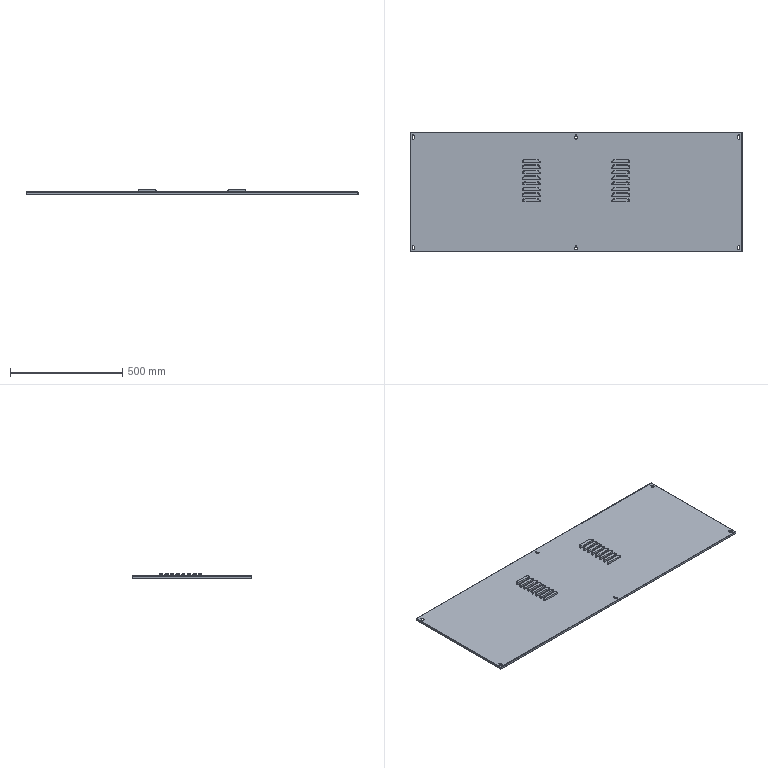Part | NX | features BREP 1 | 1 solid | 251 faces | box 1482 x 534 x 18 mm | volume 1376034 mm3 | cylinder 112 | plane 103 | torus 32 | sphere 4 | commonest cylinder face diameters 6 x54 28 x32 12 x18 2 x8